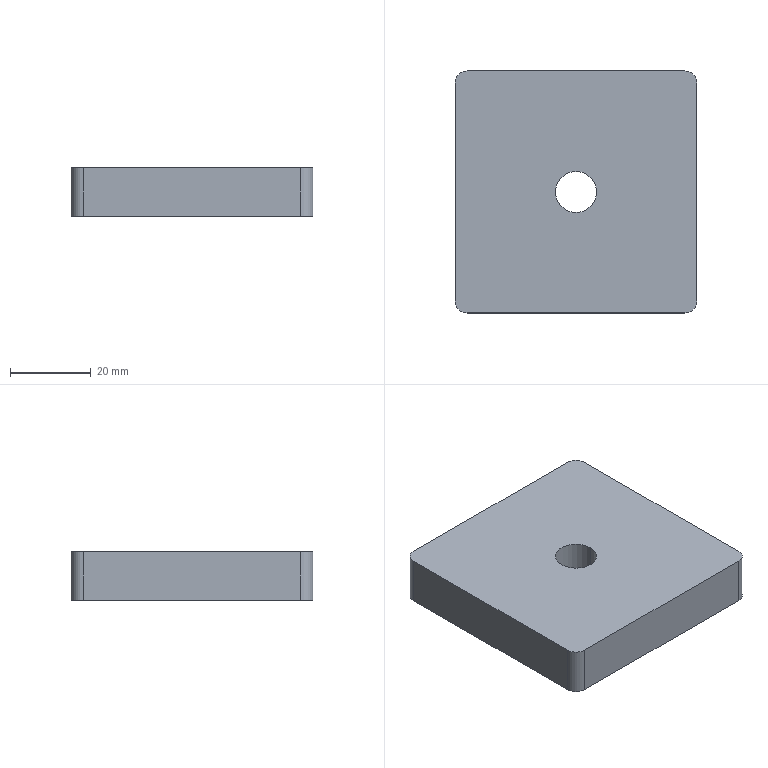Part | STEP file | X77-03103 | 1 solid | 12 faces | box 60 x 60 x 12 mm | volume 42127 mm3 | cylinder 6 | plane 6 | commonest cylinder face diameters 6 x4 10.2 x2
STEP:
#1=CARTESIAN_POINT('',(24.9,30.,0.));
#2=VERTEX_POINT('',#1);
#3=CARTESIAN_POINT('',(35.1,30.,0.));
#4=VERTEX_POINT('',#3);
#5=CARTESIAN_POINT('',(30.,30.,0.));
#6=DIRECTION('',(0.,0.,1.));
#7=DIRECTION('',(1.,0.,0.));
#8=AXIS2_PLACEMENT_3D('',#5,#6,#7);
#9=CIRCLE('',#8,5.1);
#10=EDGE_CURVE('',#2,#4,#9,.T.);
#11=ORIENTED_EDGE('',*,*,#10,.F.);
#12=CARTESIAN_POINT('',(24.9,30.,12.));
#13=VERTEX_POINT('',#12);
#14=CARTESIAN_POINT('',(24.9,30.,12.));
#15=DIRECTION('',(0.,0.,1.));
#16=VECTOR('',#15,1000.);
#17=LINE('',#14,#16);
#18=EDGE_CURVE('',#2,#13,#17,.T.);
#19=ORIENTED_EDGE('',*,*,#18,.T.);
#20=CARTESIAN_POINT('',(35.1,30.,12.));
#21=VERTEX_POINT('',#20);
#22=CARTESIAN_POINT('',(30.,30.,12.));
#23=DIRECTION('',(0.,0.,1.));
#24=DIRECTION('',(1.,0.,0.));
#25=AXIS2_PLACEMENT_3D('',#22,#23,#24);
#26=CIRCLE('',#25,5.1);
#27=EDGE_CURVE('',#13,#21,#26,.T.);
#28=ORIENTED_EDGE('',*,*,#27,.T.);
#29=CARTESIAN_POINT('',(35.1,30.,12.));
#30=DIRECTION('',(0.,0.,1.));
#31=VECTOR('',#30,1000.);
#32=LINE('',#29,#31);
#33=EDGE_CURVE('',#4,#21,#32,.T.);
#34=ORIENTED_EDGE('',*,*,#33,.F.);
#35=EDGE_LOOP('',(#11,#19,#28,#34));
#36=FACE_OUTER_BOUND('',#35,.T.);
#37=CARTESIAN_POINT('',(30.,30.,12.));
#38=DIRECTION('',(0.,0.,1.));
#39=DIRECTION('',(1.,0.,0.));
#40=AXIS2_PLACEMENT_3D('',#37,#38,#39);
#41=CYLINDRICAL_SURFACE('',#40,5.1);
#42=ADVANCED_FACE('',(#36),#41,.F.);
#43=CARTESIAN_POINT('',(0.,3.,0.));
#44=VERTEX_POINT('',#43);
#45=CARTESIAN_POINT('',(3.,0.,0.));
#46=VERTEX_POINT('',#45);
#47=CARTESIAN_POINT('',(3.,3.,0.));
#48=DIRECTION('',(0.,0.,1.));
#49=DIRECTION('',(1.,0.,0.));
#50=AXIS2_PLACEMENT_3D('',#47,#48,#49);
#51=CIRCLE('',#50,3.);
#52=EDGE_CURVE('',#44,#46,#51,.T.);
#53=ORIENTED_EDGE('',*,*,#52,.T.);
#54=CARTESIAN_POINT('',(3.,0.,12.));
#55=VERTEX_POINT('',#54);
#56=CARTESIAN_POINT('',(3.,0.,12.));
#57=DIRECTION('',(0.,0.,-1.));
#58=VECTOR('',#57,1000.);
#59=LINE('',#56,#58);
#60=EDGE_CURVE('',#55,#46,#59,.T.);
#61=ORIENTED_EDGE('',*,*,#60,.F.);
#62=CARTESIAN_POINT('',(0.,3.,12.));
#63=VERTEX_POINT('',#62);
#64=CARTESIAN_POINT('',(3.,3.,12.));
#65=DIRECTION('',(0.,0.,1.));
#66=DIRECTION('',(1.,0.,0.));
#67=AXIS2_PLACEMENT_3D('',#64,#65,#66);
#68=CIRCLE('',#67,3.);
#69=EDGE_CURVE('',#63,#55,#68,.T.);
#70=ORIENTED_EDGE('',*,*,#69,.F.);
#71=CARTESIAN_POINT('',(0.,3.,12.));
#72=DIRECTION('',(0.,0.,-1.));
#73=VECTOR('',#72,1000.);
#74=LINE('',#71,#73);
#75=EDGE_CURVE('',#63,#44,#74,.T.);
#76=ORIENTED_EDGE('',*,*,#75,.T.);
#77=EDGE_LOOP('',(#53,#61,#70,#76));
#78=FACE_OUTER_BOUND('',#77,.T.);
#79=CARTESIAN_POINT('',(3.,3.,12.));
#80=DIRECTION('',(0.,0.,-1.));
#81=DIRECTION('',(-1.,0.,0.));
#82=AXIS2_PLACEMENT_3D('',#79,#80,#81);
#83=CYLINDRICAL_SURFACE('',#82,3.);
#84=ADVANCED_FACE('',(#78),#83,.T.);
#85=CARTESIAN_POINT('',(57.,0.,0.));
#86=VERTEX_POINT('',#85);
#87=CARTESIAN_POINT('',(3.,0.,0.));
#88=DIRECTION('',(1.,0.,0.));
#89=VECTOR('',#88,1000.);
#90=LINE('',#87,#89);
#91=EDGE_CURVE('',#46,#86,#90,.T.);
#92=ORIENTED_EDGE('',*,*,#91,.T.);
#93=CARTESIAN_POINT('',(57.,0.,12.));
#94=VERTEX_POINT('',#93);
#95=CARTESIAN_POINT('',(57.,0.,12.));
#96=DIRECTION('',(0.,0.,-1.));
#97=VECTOR('',#96,1000.);
#98=LINE('',#95,#97);
#99=EDGE_CURVE('',#94,#86,#98,.T.);
#100=ORIENTED_EDGE('',*,*,#99,.F.);
#101=CARTESIAN_POINT('',(3.,0.,12.));
#102=DIRECTION('',(1.,0.,0.));
#103=VECTOR('',#102,1000.);
#104=LINE('',#101,#103);
#105=EDGE_CURVE('',#55,#94,#104,.T.);
#106=ORIENTED_EDGE('',*,*,#105,.F.);
#107=ORIENTED_EDGE('',*,*,#60,.T.);
#108=EDGE_LOOP('',(#92,#100,#106,#107));
#109=FACE_OUTER_BOUND('',#108,.T.);
#110=CARTESIAN_POINT('',(3.,0.,12.));
#111=DIRECTION('',(0.,1.,0.));
#112=DIRECTION('',(0.,0.,1.));
#113=AXIS2_PLACEMENT_3D('',#110,#111,#112);
#114=PLANE('',#113);
#115=ADVANCED_FACE('',(#109),#114,.F.);
#116=CARTESIAN_POINT('',(60.,3.,0.));
#117=VERTEX_POINT('',#116);
#118=CARTESIAN_POINT('',(57.,3.,0.));
#119=DIRECTION('',(0.,0.,1.));
#120=DIRECTION('',(1.,0.,0.));
#121=AXIS2_PLACEMENT_3D('',#118,#119,#120);
#122=CIRCLE('',#121,3.);
#123=EDGE_CURVE('',#86,#117,#122,.T.);
#124=ORIENTED_EDGE('',*,*,#123,.T.);
#125=CARTESIAN_POINT('',(60.,3.,12.));
#126=VERTEX_POINT('',#125);
#127=CARTESIAN_POINT('',(60.,3.,12.));
#128=DIRECTION('',(0.,0.,-1.));
#129=VECTOR('',#128,1000.);
#130=LINE('',#127,#129);
#131=EDGE_CURVE('',#126,#117,#130,.T.);
#132=ORIENTED_EDGE('',*,*,#131,.F.);
#133=CARTESIAN_POINT('',(57.,3.,12.));
#134=DIRECTION('',(0.,0.,1.));
#135=DIRECTION('',(1.,0.,0.));
#136=AXIS2_PLACEMENT_3D('',#133,#134,#135);
#137=CIRCLE('',#136,3.);
#138=EDGE_CURVE('',#94,#126,#137,.T.);
#139=ORIENTED_EDGE('',*,*,#138,.F.);
#140=ORIENTED_EDGE('',*,*,#99,.T.);
#141=EDGE_LOOP('',(#124,#132,#139,#140));
#142=FACE_OUTER_BOUND('',#141,.T.);
#143=CARTESIAN_POINT('',(57.,3.,12.));
#144=DIRECTION('',(0.,0.,-1.));
#145=DIRECTION('',(-1.,0.,0.));
#146=AXIS2_PLACEMENT_3D('',#143,#144,#145);
#147=CYLINDRICAL_SURFACE('',#146,3.);
#148=ADVANCED_FACE('',(#142),#147,.T.);
#149=CARTESIAN_POINT('',(60.,57.,0.));
#150=VERTEX_POINT('',#149);
#151=CARTESIAN_POINT('',(60.,3.,0.));
#152=DIRECTION('',(0.,1.,0.));
#153=VECTOR('',#152,1000.);
#154=LINE('',#151,#153);
#155=EDGE_CURVE('',#117,#150,#154,.T.);
#156=ORIENTED_EDGE('',*,*,#155,.T.);
#157=CARTESIAN_POINT('',(60.,57.,12.));
#158=VERTEX_POINT('',#157);
#159=CARTESIAN_POINT('',(60.,57.,12.));
#160=DIRECTION('',(0.,0.,-1.));
#161=VECTOR('',#160,1000.);
#162=LINE('',#159,#161);
#163=EDGE_CURVE('',#158,#150,#162,.T.);
#164=ORIENTED_EDGE('',*,*,#163,.F.);
#165=CARTESIAN_POINT('',(60.,3.,12.));
#166=DIRECTION('',(0.,1.,0.));
#167=VECTOR('',#166,1000.);
#168=LINE('',#165,#167);
#169=EDGE_CURVE('',#126,#158,#168,.T.);
#170=ORIENTED_EDGE('',*,*,#169,.F.);
#171=ORIENTED_EDGE('',*,*,#131,.T.);
#172=EDGE_LOOP('',(#156,#164,#170,#171));
#173=FACE_OUTER_BOUND('',#172,.T.);
#174=CARTESIAN_POINT('',(60.,3.,12.));
#175=DIRECTION('',(-1.,0.,0.));
#176=DIRECTION('',(0.,0.,1.));
#177=AXIS2_PLACEMENT_3D('',#174,#175,#176);
#178=PLANE('',#177);
#179=ADVANCED_FACE('',(#173),#178,.F.);
#180=CARTESIAN_POINT('',(57.,60.,0.));
#181=VERTEX_POINT('',#180);
#182=CARTESIAN_POINT('',(57.,57.,0.));
#183=DIRECTION('',(0.,0.,1.));
#184=DIRECTION('',(1.,0.,0.));
#185=AXIS2_PLACEMENT_3D('',#182,#183,#184);
#186=CIRCLE('',#185,3.);
#187=EDGE_CURVE('',#150,#181,#186,.T.);
#188=ORIENTED_EDGE('',*,*,#187,.T.);
#189=CARTESIAN_POINT('',(57.,60.,12.));
#190=VERTEX_POINT('',#189);
#191=CARTESIAN_POINT('',(57.,60.,12.));
#192=DIRECTION('',(0.,0.,-1.));
#193=VECTOR('',#192,1000.);
#194=LINE('',#191,#193);
#195=EDGE_CURVE('',#190,#181,#194,.T.);
#196=ORIENTED_EDGE('',*,*,#195,.F.);
#197=CARTESIAN_POINT('',(57.,57.,12.));
#198=DIRECTION('',(0.,0.,1.));
#199=DIRECTION('',(1.,0.,0.));
#200=AXIS2_PLACEMENT_3D('',#197,#198,#199);
#201=CIRCLE('',#200,3.);
#202=EDGE_CURVE('',#158,#190,#201,.T.);
#203=ORIENTED_EDGE('',*,*,#202,.F.);
#204=ORIENTED_EDGE('',*,*,#163,.T.);
#205=EDGE_LOOP('',(#188,#196,#203,#204));
#206=FACE_OUTER_BOUND('',#205,.T.);
#207=CARTESIAN_POINT('',(57.,57.,12.));
#208=DIRECTION('',(0.,0.,-1.));
#209=DIRECTION('',(-1.,0.,0.));
#210=AXIS2_PLACEMENT_3D('',#207,#208,#209);
#211=CYLINDRICAL_SURFACE('',#210,3.);
#212=ADVANCED_FACE('',(#206),#211,.T.);
#213=CARTESIAN_POINT('',(3.,60.,0.));
#214=VERTEX_POINT('',#213);
#215=CARTESIAN_POINT('',(3.,60.,0.));
#216=DIRECTION('',(-1.,0.,0.));
#217=VECTOR('',#216,1000.);
#218=LINE('',#215,#217);
#219=EDGE_CURVE('',#181,#214,#218,.T.);
#220=ORIENTED_EDGE('',*,*,#219,.T.);
#221=CARTESIAN_POINT('',(3.,60.,12.));
#222=VERTEX_POINT('',#221);
#223=CARTESIAN_POINT('',(3.,60.,12.));
#224=DIRECTION('',(0.,0.,-1.));
#225=VECTOR('',#224,1000.);
#226=LINE('',#223,#225);
#227=EDGE_CURVE('',#222,#214,#226,.T.);
#228=ORIENTED_EDGE('',*,*,#227,.F.);
#229=CARTESIAN_POINT('',(3.,60.,12.));
#230=DIRECTION('',(-1.,0.,0.));
#231=VECTOR('',#230,1000.);
#232=LINE('',#229,#231);
#233=EDGE_CURVE('',#190,#222,#232,.T.);
#234=ORIENTED_EDGE('',*,*,#233,.F.);
#235=ORIENTED_EDGE('',*,*,#195,.T.);
#236=EDGE_LOOP('',(#220,#228,#234,#235));
#237=FACE_OUTER_BOUND('',#236,.T.);
#238=CARTESIAN_POINT('',(3.,60.,12.));
#239=DIRECTION('',(0.,-1.,0.));
#240=DIRECTION('',(0.,0.,-1.));
#241=AXIS2_PLACEMENT_3D('',#238,#239,#240);
#242=PLANE('',#241);
#243=ADVANCED_FACE('',(#237),#242,.F.);
#244=CARTESIAN_POINT('',(0.,57.,0.));
#245=VERTEX_POINT('',#244);
#246=CARTESIAN_POINT('',(3.,57.,0.));
#247=DIRECTION('',(0.,0.,1.));
#248=DIRECTION('',(-1.,0.,0.));
#249=AXIS2_PLACEMENT_3D('',#246,#247,#248);
#250=CIRCLE('',#249,3.);
#251=EDGE_CURVE('',#214,#245,#250,.T.);
#252=ORIENTED_EDGE('',*,*,#251,.T.);
#253=CARTESIAN_POINT('',(0.,57.,12.));
#254=VERTEX_POINT('',#253);
#255=CARTESIAN_POINT('',(0.,57.,12.));
#256=DIRECTION('',(0.,0.,-1.));
#257=VECTOR('',#256,1000.);
#258=LINE('',#255,#257);
#259=EDGE_CURVE('',#254,#245,#258,.T.);
#260=ORIENTED_EDGE('',*,*,#259,.F.);
#261=CARTESIAN_POINT('',(3.,57.,12.));
#262=DIRECTION('',(0.,0.,1.));
#263=DIRECTION('',(-1.,0.,0.));
#264=AXIS2_PLACEMENT_3D('',#261,#262,#263);
#265=CIRCLE('',#264,3.);
#266=EDGE_CURVE('',#222,#254,#265,.T.);
#267=ORIENTED_EDGE('',*,*,#266,.F.);
#268=ORIENTED_EDGE('',*,*,#227,.T.);
#269=EDGE_LOOP('',(#252,#260,#267,#268));
#270=FACE_OUTER_BOUND('',#269,.T.);
#271=CARTESIAN_POINT('',(3.,57.,12.));
#272=DIRECTION('',(0.,0.,-1.));
#273=DIRECTION('',(-1.,0.,0.));
#274=AXIS2_PLACEMENT_3D('',#271,#272,#273);
#275=CYLINDRICAL_SURFACE('',#274,3.);
#276=ADVANCED_FACE('',(#270),#275,.T.);
#277=CARTESIAN_POINT('',(0.,3.,0.));
#278=DIRECTION('',(0.,-1.,0.));
#279=VECTOR('',#278,1000.);
#280=LINE('',#277,#279);
#281=EDGE_CURVE('',#245,#44,#280,.T.);
#282=ORIENTED_EDGE('',*,*,#281,.T.);
#283=ORIENTED_EDGE('',*,*,#75,.F.);
#284=CARTESIAN_POINT('',(0.,3.,12.));
#285=DIRECTION('',(0.,-1.,0.));
#286=VECTOR('',#285,1000.);
#287=LINE('',#284,#286);
#288=EDGE_CURVE('',#254,#63,#287,.T.);
#289=ORIENTED_EDGE('',*,*,#288,.F.);
#290=ORIENTED_EDGE('',*,*,#259,.T.);
#291=EDGE_LOOP('',(#282,#283,#289,#290));
#292=FACE_OUTER_BOUND('',#291,.T.);
#293=CARTESIAN_POINT('',(0.,3.,12.));
#294=DIRECTION('',(1.,0.,0.));
#295=DIRECTION('',(0.,0.,-1.));
#296=AXIS2_PLACEMENT_3D('',#293,#294,#295);
#297=PLANE('',#296);
#298=ADVANCED_FACE('',(#292),#297,.F.);
#299=CARTESIAN_POINT('',(30.,30.,12.));
#300=DIRECTION('',(0.,0.,1.));
#301=DIRECTION('',(1.,0.,0.));
#302=AXIS2_PLACEMENT_3D('',#299,#300,#301);
#303=CIRCLE('',#302,5.1);
#304=EDGE_CURVE('',#21,#13,#303,.T.);
#305=ORIENTED_EDGE('',*,*,#304,.F.);
#306=ORIENTED_EDGE('',*,*,#27,.F.);
#307=EDGE_LOOP('',(#305,#306));
#308=FACE_BOUND('',#307,.T.);
#309=ORIENTED_EDGE('',*,*,#69,.T.);
#310=ORIENTED_EDGE('',*,*,#105,.T.);
#311=ORIENTED_EDGE('',*,*,#138,.T.);
#312=ORIENTED_EDGE('',*,*,#169,.T.);
#313=ORIENTED_EDGE('',*,*,#202,.T.);
#314=ORIENTED_EDGE('',*,*,#233,.T.);
#315=ORIENTED_EDGE('',*,*,#266,.T.);
#316=ORIENTED_EDGE('',*,*,#288,.T.);
#317=EDGE_LOOP('',(#309,#310,#311,#312,#313,#314,#315,#316));
#318=FACE_OUTER_BOUND('',#317,.T.);
#319=CARTESIAN_POINT('',(3.,3.,12.));
#320=DIRECTION('',(0.,0.,1.));
#321=DIRECTION('',(1.,0.,0.));
#322=AXIS2_PLACEMENT_3D('',#319,#320,#321);
#323=PLANE('',#322);
#324=ADVANCED_FACE('',(#308,#318),#323,.T.);
#325=CARTESIAN_POINT('',(30.,30.,0.));
#326=DIRECTION('',(0.,0.,1.));
#327=DIRECTION('',(1.,0.,0.));
#328=AXIS2_PLACEMENT_3D('',#325,#326,#327);
#329=CIRCLE('',#328,5.1);
#330=EDGE_CURVE('',#4,#2,#329,.T.);
#331=ORIENTED_EDGE('',*,*,#330,.T.);
#332=ORIENTED_EDGE('',*,*,#10,.T.);
#333=EDGE_LOOP('',(#331,#332));
#334=FACE_BOUND('',#333,.T.);
#335=ORIENTED_EDGE('',*,*,#52,.F.);
#336=ORIENTED_EDGE('',*,*,#281,.F.);
#337=ORIENTED_EDGE('',*,*,#251,.F.);
#338=ORIENTED_EDGE('',*,*,#219,.F.);
#339=ORIENTED_EDGE('',*,*,#187,.F.);
#340=ORIENTED_EDGE('',*,*,#155,.F.);
#341=ORIENTED_EDGE('',*,*,#123,.F.);
#342=ORIENTED_EDGE('',*,*,#91,.F.);
#343=EDGE_LOOP('',(#335,#336,#337,#338,#339,#340,#341,#342));
#344=FACE_OUTER_BOUND('',#343,.T.);
#345=CARTESIAN_POINT('',(3.,3.,0.));
#346=DIRECTION('',(0.,0.,1.));
#347=DIRECTION('',(1.,0.,0.));
#348=AXIS2_PLACEMENT_3D('',#345,#346,#347);
#349=PLANE('',#348);
#350=ADVANCED_FACE('',(#334,#344),#349,.F.);
#351=ORIENTED_EDGE('',*,*,#18,.F.);
#352=ORIENTED_EDGE('',*,*,#330,.F.);
#353=ORIENTED_EDGE('',*,*,#33,.T.);
#354=ORIENTED_EDGE('',*,*,#304,.T.);
#355=EDGE_LOOP('',(#351,#352,#353,#354));
#356=FACE_OUTER_BOUND('',#355,.T.);
#357=CARTESIAN_POINT('',(30.,30.,12.));
#358=DIRECTION('',(0.,0.,1.));
#359=DIRECTION('',(1.,0.,0.));
#360=AXIS2_PLACEMENT_3D('',#357,#358,#359);
#361=CYLINDRICAL_SURFACE('',#360,5.1);
#362=ADVANCED_FACE('',(#356),#361,.F.);
#363=CLOSED_SHELL('',(#42,#84,#115,#148,#179,#212,#243,#276,#298,#324,#350,#362));
#364=MANIFOLD_SOLID_BREP('',#363);
#365=CARTESIAN_POINT('',(0.,0.,0.));
#366=DIRECTION('',(0.,0.,1.));
#367=DIRECTION('',(1.,0.,0.));
#368=AXIS2_PLACEMENT_3D('',#365,#366,#367);
#369=(LENGTH_UNIT()NAMED_UNIT(*)SI_UNIT(.MILLI.,.METRE.));
#370=UNCERTAINTY_MEASURE_WITH_UNIT(LENGTH_MEASURE(0.00001),#369,'','');
#371=(NAMED_UNIT(*)PLANE_ANGLE_UNIT()SI_UNIT($,.RADIAN.));
#372=(NAMED_UNIT(*)SI_UNIT($,.STERADIAN.)SOLID_ANGLE_UNIT());
#373=(GEOMETRIC_REPRESENTATION_CONTEXT(3)GLOBAL_UNCERTAINTY_ASSIGNED_CONTEXT((#370))GLOBAL_UNIT_ASSIGNED_CONTEXT((#369,#371,#372))REPRESENTATION_CONTEXT('',''));
#374=ADVANCED_BREP_SHAPE_REPRESENTATION('',(#364,#368),#373);